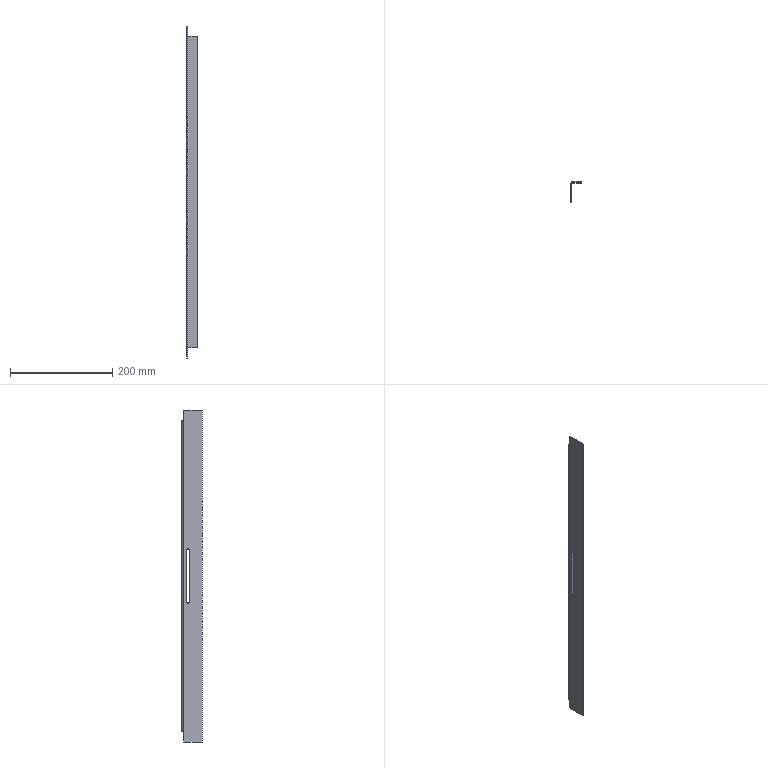Part | SolidWorks | features SMBaseFlange 2, FlatPattern 1, ICE 1, SheetMetal 1 | 1 solid | 21 faces | box 20 x 40 x 649 mm | volume 70699 mm3 | plane 16 | cylinder 5 | commonest cylinder face diameters 6 x3 4 x1 8 x1
STEP:
#1=CARTESIAN_POINT('',(0.,28.,251.5));
#2=VERTEX_POINT('',#1);
#3=CARTESIAN_POINT('',(0.,31.,254.5));
#4=VERTEX_POINT('',#3);
#5=CARTESIAN_POINT('',(0.,28.,254.5));
#6=DIRECTION('',(1.,0.,0.));
#7=DIRECTION('',(0.,0.,-1.));
#8=AXIS2_PLACEMENT_3D('',#5,#6,#7);
#9=CIRCLE('',#8,3.);
#10=EDGE_CURVE('',#2,#4,#9,.T.);
#11=ORIENTED_EDGE('',*,*,#10,.F.);
#12=CARTESIAN_POINT('',(2.,28.,251.5));
#13=VERTEX_POINT('',#12);
#14=CARTESIAN_POINT('',(0.,28.,251.5));
#15=DIRECTION('',(1.,0.,0.));
#16=VECTOR('',#15,1000.);
#17=LINE('',#14,#16);
#18=EDGE_CURVE('',#2,#13,#17,.T.);
#19=ORIENTED_EDGE('',*,*,#18,.T.);
#20=CARTESIAN_POINT('',(2.,31.,254.5));
#21=VERTEX_POINT('',#20);
#22=CARTESIAN_POINT('',(2.,28.,254.5));
#23=DIRECTION('',(1.,0.,0.));
#24=DIRECTION('',(0.,0.,-1.));
#25=AXIS2_PLACEMENT_3D('',#22,#23,#24);
#26=CIRCLE('',#25,3.);
#27=EDGE_CURVE('',#13,#21,#26,.T.);
#28=ORIENTED_EDGE('',*,*,#27,.T.);
#29=CARTESIAN_POINT('',(0.,31.,254.5));
#30=DIRECTION('',(1.,0.,0.));
#31=VECTOR('',#30,1000.);
#32=LINE('',#29,#31);
#33=EDGE_CURVE('',#4,#21,#32,.T.);
#34=ORIENTED_EDGE('',*,*,#33,.F.);
#35=EDGE_LOOP('',(#11,#19,#28,#34));
#36=FACE_OUTER_BOUND('',#35,.T.);
#37=CARTESIAN_POINT('',(0.,28.,254.5));
#38=DIRECTION('',(1.,0.,0.));
#39=DIRECTION('',(0.,0.,-1.));
#40=AXIS2_PLACEMENT_3D('',#37,#38,#39);
#41=CYLINDRICAL_SURFACE('',#40,3.);
#42=ADVANCED_FACE('',(#36),#41,.F.);
#43=CARTESIAN_POINT('',(4.,40.,609.));
#44=VERTEX_POINT('',#43);
#45=CARTESIAN_POINT('',(4.,38.,609.));
#46=VERTEX_POINT('',#45);
#47=CARTESIAN_POINT('',(4.,40.,609.));
#48=DIRECTION('',(0.,-1.,0.));
#49=VECTOR('',#48,1000.);
#50=LINE('',#47,#49);
#51=EDGE_CURVE('',#44,#46,#50,.T.);
#52=ORIENTED_EDGE('',*,*,#51,.F.);
#53=CARTESIAN_POINT('',(0.,36.,609.));
#54=VERTEX_POINT('',#53);
#55=CARTESIAN_POINT('',(4.,36.,609.));
#56=DIRECTION('',(0.,0.,-1.));
#57=DIRECTION('',(1.,0.,0.));
#58=AXIS2_PLACEMENT_3D('',#55,#56,#57);
#59=CIRCLE('',#58,4.);
#60=EDGE_CURVE('',#54,#44,#59,.T.);
#61=ORIENTED_EDGE('',*,*,#60,.F.);
#62=CARTESIAN_POINT('',(2.,36.,609.));
#63=VERTEX_POINT('',#62);
#64=CARTESIAN_POINT('',(2.,36.,609.));
#65=DIRECTION('',(-1.,0.,0.));
#66=VECTOR('',#65,1000.);
#67=LINE('',#64,#66);
#68=EDGE_CURVE('',#63,#54,#67,.T.);
#69=ORIENTED_EDGE('',*,*,#68,.F.);
#70=CARTESIAN_POINT('',(4.,36.,609.));
#71=DIRECTION('',(0.,0.,-1.));
#72=DIRECTION('',(1.,0.,0.));
#73=AXIS2_PLACEMENT_3D('',#70,#71,#72);
#74=CIRCLE('',#73,2.);
#75=EDGE_CURVE('',#63,#46,#74,.T.);
#76=ORIENTED_EDGE('',*,*,#75,.T.);
#77=EDGE_LOOP('',(#52,#61,#69,#76));
#78=FACE_OUTER_BOUND('',#77,.T.);
#79=CARTESIAN_POINT('',(4.,40.,609.));
#80=DIRECTION('',(0.,0.,1.));
#81=DIRECTION('',(1.,0.,0.));
#82=AXIS2_PLACEMENT_3D('',#79,#80,#81);
#83=PLANE('',#82);
#84=ADVANCED_FACE('',(#78),#83,.T.);
#85=CARTESIAN_POINT('',(20.,40.,609.));
#86=VERTEX_POINT('',#85);
#87=CARTESIAN_POINT('',(0.,40.,609.));
#88=DIRECTION('',(1.,0.,0.));
#89=VECTOR('',#88,1000.);
#90=LINE('',#87,#89);
#91=EDGE_CURVE('',#44,#86,#90,.T.);
#92=ORIENTED_EDGE('',*,*,#91,.F.);
#93=ORIENTED_EDGE('',*,*,#51,.T.);
#94=CARTESIAN_POINT('',(20.,38.,609.));
#95=VERTEX_POINT('',#94);
#96=CARTESIAN_POINT('',(0.,38.,609.));
#97=DIRECTION('',(1.,0.,0.));
#98=VECTOR('',#97,1000.);
#99=LINE('',#96,#98);
#100=EDGE_CURVE('',#46,#95,#99,.T.);
#101=ORIENTED_EDGE('',*,*,#100,.T.);
#102=CARTESIAN_POINT('',(20.,40.,609.));
#103=DIRECTION('',(0.,-1.,0.));
#104=VECTOR('',#103,1000.);
#105=LINE('',#102,#104);
#106=EDGE_CURVE('',#86,#95,#105,.T.);
#107=ORIENTED_EDGE('',*,*,#106,.F.);
#108=EDGE_LOOP('',(#92,#93,#101,#107));
#109=FACE_OUTER_BOUND('',#108,.T.);
#110=CARTESIAN_POINT('',(2.,36.,609.));
#111=DIRECTION('',(0.,0.,1.));
#112=DIRECTION('',(1.,0.,0.));
#113=AXIS2_PLACEMENT_3D('',#110,#111,#112);
#114=PLANE('',#113);
#115=ADVANCED_FACE('',(#109),#114,.T.);
#116=CARTESIAN_POINT('',(0.,36.,0.));
#117=VERTEX_POINT('',#116);
#118=CARTESIAN_POINT('',(2.,36.,0.));
#119=VERTEX_POINT('',#118);
#120=CARTESIAN_POINT('',(0.,36.,0.));
#121=DIRECTION('',(1.,0.,0.));
#122=VECTOR('',#121,1000.);
#123=LINE('',#120,#122);
#124=EDGE_CURVE('',#117,#119,#123,.T.);
#125=ORIENTED_EDGE('',*,*,#124,.F.);
#126=CARTESIAN_POINT('',(4.,40.,0.));
#127=VERTEX_POINT('',#126);
#128=CARTESIAN_POINT('',(4.,36.,0.));
#129=DIRECTION('',(0.,0.,-1.));
#130=DIRECTION('',(1.,0.,0.));
#131=AXIS2_PLACEMENT_3D('',#128,#129,#130);
#132=CIRCLE('',#131,4.);
#133=EDGE_CURVE('',#117,#127,#132,.T.);
#134=ORIENTED_EDGE('',*,*,#133,.T.);
#135=CARTESIAN_POINT('',(4.,38.,0.));
#136=VERTEX_POINT('',#135);
#137=CARTESIAN_POINT('',(4.,38.,0.));
#138=DIRECTION('',(0.,1.,0.));
#139=VECTOR('',#138,1000.);
#140=LINE('',#137,#139);
#141=EDGE_CURVE('',#136,#127,#140,.T.);
#142=ORIENTED_EDGE('',*,*,#141,.F.);
#143=CARTESIAN_POINT('',(4.,36.,0.));
#144=DIRECTION('',(0.,0.,-1.));
#145=DIRECTION('',(1.,0.,0.));
#146=AXIS2_PLACEMENT_3D('',#143,#144,#145);
#147=CIRCLE('',#146,2.);
#148=EDGE_CURVE('',#119,#136,#147,.T.);
#149=ORIENTED_EDGE('',*,*,#148,.F.);
#150=EDGE_LOOP('',(#125,#134,#142,#149));
#151=FACE_OUTER_BOUND('',#150,.T.);
#152=CARTESIAN_POINT('',(0.,36.,0.));
#153=DIRECTION('',(0.,0.,-1.));
#154=DIRECTION('',(-1.,0.,0.));
#155=AXIS2_PLACEMENT_3D('',#152,#153,#154);
#156=PLANE('',#155);
#157=ADVANCED_FACE('',(#151),#156,.T.);
#158=CARTESIAN_POINT('',(20.,38.,0.));
#159=VERTEX_POINT('',#158);
#160=CARTESIAN_POINT('',(0.,38.,0.));
#161=DIRECTION('',(1.,0.,0.));
#162=VECTOR('',#161,1000.);
#163=LINE('',#160,#162);
#164=EDGE_CURVE('',#136,#159,#163,.T.);
#165=ORIENTED_EDGE('',*,*,#164,.T.);
#166=CARTESIAN_POINT('',(20.,38.,609.));
#167=DIRECTION('',(0.,0.,-1.));
#168=VECTOR('',#167,1000.);
#169=LINE('',#166,#168);
#170=EDGE_CURVE('',#95,#159,#169,.T.);
#171=ORIENTED_EDGE('',*,*,#170,.F.);
#172=ORIENTED_EDGE('',*,*,#100,.F.);
#173=CARTESIAN_POINT('',(4.,38.,609.));
#174=DIRECTION('',(0.,0.,-1.));
#175=VECTOR('',#174,1000.);
#176=LINE('',#173,#175);
#177=EDGE_CURVE('',#46,#136,#176,.T.);
#178=ORIENTED_EDGE('',*,*,#177,.T.);
#179=EDGE_LOOP('',(#165,#171,#172,#178));
#180=FACE_OUTER_BOUND('',#179,.T.);
#181=CARTESIAN_POINT('',(0.,38.,609.));
#182=DIRECTION('',(0.,1.,0.));
#183=DIRECTION('',(0.,0.,1.));
#184=AXIS2_PLACEMENT_3D('',#181,#182,#183);
#185=PLANE('',#184);
#186=ADVANCED_FACE('',(#180),#185,.F.);
#187=CARTESIAN_POINT('',(20.,40.,0.));
#188=VERTEX_POINT('',#187);
#189=CARTESIAN_POINT('',(20.,40.,0.));
#190=DIRECTION('',(0.,-1.,0.));
#191=VECTOR('',#190,1000.);
#192=LINE('',#189,#191);
#193=EDGE_CURVE('',#188,#159,#192,.T.);
#194=ORIENTED_EDGE('',*,*,#193,.F.);
#195=CARTESIAN_POINT('',(20.,40.,609.));
#196=DIRECTION('',(0.,0.,-1.));
#197=VECTOR('',#196,1000.);
#198=LINE('',#195,#197);
#199=EDGE_CURVE('',#86,#188,#198,.T.);
#200=ORIENTED_EDGE('',*,*,#199,.F.);
#201=ORIENTED_EDGE('',*,*,#106,.T.);
#202=ORIENTED_EDGE('',*,*,#170,.T.);
#203=EDGE_LOOP('',(#194,#200,#201,#202));
#204=FACE_OUTER_BOUND('',#203,.T.);
#205=CARTESIAN_POINT('',(20.,40.,609.));
#206=DIRECTION('',(1.,0.,0.));
#207=DIRECTION('',(0.,0.,-1.));
#208=AXIS2_PLACEMENT_3D('',#205,#206,#207);
#209=PLANE('',#208);
#210=ADVANCED_FACE('',(#204),#209,.T.);
#211=CARTESIAN_POINT('',(0.,40.,0.));
#212=DIRECTION('',(1.,0.,0.));
#213=VECTOR('',#212,1000.);
#214=LINE('',#211,#213);
#215=EDGE_CURVE('',#127,#188,#214,.T.);
#216=ORIENTED_EDGE('',*,*,#215,.F.);
#217=CARTESIAN_POINT('',(4.,40.,609.));
#218=DIRECTION('',(0.,0.,-1.));
#219=VECTOR('',#218,1000.);
#220=LINE('',#217,#219);
#221=EDGE_CURVE('',#44,#127,#220,.T.);
#222=ORIENTED_EDGE('',*,*,#221,.F.);
#223=ORIENTED_EDGE('',*,*,#91,.T.);
#224=ORIENTED_EDGE('',*,*,#199,.T.);
#225=EDGE_LOOP('',(#216,#222,#223,#224));
#226=FACE_OUTER_BOUND('',#225,.T.);
#227=CARTESIAN_POINT('',(0.,40.,609.));
#228=DIRECTION('',(0.,1.,0.));
#229=DIRECTION('',(0.,0.,1.));
#230=AXIS2_PLACEMENT_3D('',#227,#228,#229);
#231=PLANE('',#230);
#232=ADVANCED_FACE('',(#226),#231,.T.);
#233=ORIENTED_EDGE('',*,*,#133,.F.);
#234=CARTESIAN_POINT('',(0.,36.,609.));
#235=DIRECTION('',(0.,0.,-1.));
#236=VECTOR('',#235,1000.);
#237=LINE('',#234,#236);
#238=EDGE_CURVE('',#54,#117,#237,.T.);
#239=ORIENTED_EDGE('',*,*,#238,.F.);
#240=ORIENTED_EDGE('',*,*,#60,.T.);
#241=ORIENTED_EDGE('',*,*,#221,.T.);
#242=EDGE_LOOP('',(#233,#239,#240,#241));
#243=FACE_OUTER_BOUND('',#242,.T.);
#244=CARTESIAN_POINT('',(4.,36.,609.));
#245=DIRECTION('',(0.,0.,-1.));
#246=DIRECTION('',(-1.,0.,0.));
#247=AXIS2_PLACEMENT_3D('',#244,#245,#246);
#248=CYLINDRICAL_SURFACE('',#247,4.);
#249=ADVANCED_FACE('',(#243),#248,.T.);
#250=CARTESIAN_POINT('',(0.,25.,254.5));
#251=VERTEX_POINT('',#250);
#252=CARTESIAN_POINT('',(0.,28.,254.5));
#253=DIRECTION('',(1.,0.,0.));
#254=DIRECTION('',(0.,0.,-1.));
#255=AXIS2_PLACEMENT_3D('',#252,#253,#254);
#256=CIRCLE('',#255,3.);
#257=EDGE_CURVE('',#251,#2,#256,.T.);
#258=ORIENTED_EDGE('',*,*,#257,.T.);
#259=ORIENTED_EDGE('',*,*,#10,.T.);
#260=CARTESIAN_POINT('',(0.,31.,354.5));
#261=VERTEX_POINT('',#260);
#262=CARTESIAN_POINT('',(0.,31.,254.5));
#263=DIRECTION('',(0.,0.,1.));
#264=VECTOR('',#263,1000.);
#265=LINE('',#262,#264);
#266=EDGE_CURVE('',#4,#261,#265,.T.);
#267=ORIENTED_EDGE('',*,*,#266,.T.);
#268=CARTESIAN_POINT('',(0.,25.,354.5));
#269=VERTEX_POINT('',#268);
#270=CARTESIAN_POINT('',(0.,28.,354.5));
#271=DIRECTION('',(1.,0.,0.));
#272=DIRECTION('',(0.,0.,-1.));
#273=AXIS2_PLACEMENT_3D('',#270,#271,#272);
#274=CIRCLE('',#273,3.);
#275=EDGE_CURVE('',#261,#269,#274,.T.);
#276=ORIENTED_EDGE('',*,*,#275,.T.);
#277=CARTESIAN_POINT('',(0.,25.,254.5));
#278=DIRECTION('',(0.,0.,-1.));
#279=VECTOR('',#278,1000.);
#280=LINE('',#277,#279);
#281=EDGE_CURVE('',#269,#251,#280,.T.);
#282=ORIENTED_EDGE('',*,*,#281,.T.);
#283=EDGE_LOOP('',(#258,#259,#267,#276,#282));
#284=FACE_BOUND('',#283,.T.);
#285=ORIENTED_EDGE('',*,*,#238,.T.);
#286=CARTESIAN_POINT('',(0.,36.,-20.));
#287=VERTEX_POINT('',#286);
#288=CARTESIAN_POINT('',(0.,36.,0.));
#289=DIRECTION('',(0.,0.,1.));
#290=VECTOR('',#289,1000.);
#291=LINE('',#288,#290);
#292=EDGE_CURVE('',#287,#117,#291,.T.);
#293=ORIENTED_EDGE('',*,*,#292,.F.);
#294=CARTESIAN_POINT('',(0.,0.,-20.));
#295=VERTEX_POINT('',#294);
#296=CARTESIAN_POINT('',(0.,0.,-20.));
#297=DIRECTION('',(0.,1.,0.));
#298=VECTOR('',#297,1000.);
#299=LINE('',#296,#298);
#300=EDGE_CURVE('',#295,#287,#299,.T.);
#301=ORIENTED_EDGE('',*,*,#300,.F.);
#302=CARTESIAN_POINT('',(0.,0.,629.));
#303=VERTEX_POINT('',#302);
#304=CARTESIAN_POINT('',(0.,0.,609.));
#305=DIRECTION('',(0.,0.,-1.));
#306=VECTOR('',#305,1000.);
#307=LINE('',#304,#306);
#308=EDGE_CURVE('',#303,#295,#307,.T.);
#309=ORIENTED_EDGE('',*,*,#308,.F.);
#310=CARTESIAN_POINT('',(0.,36.,629.));
#311=VERTEX_POINT('',#310);
#312=CARTESIAN_POINT('',(0.,0.,629.));
#313=DIRECTION('',(0.,-1.,0.));
#314=VECTOR('',#313,1000.);
#315=LINE('',#312,#314);
#316=EDGE_CURVE('',#311,#303,#315,.T.);
#317=ORIENTED_EDGE('',*,*,#316,.F.);
#318=CARTESIAN_POINT('',(0.,36.,609.));
#319=DIRECTION('',(0.,0.,1.));
#320=VECTOR('',#319,1000.);
#321=LINE('',#318,#320);
#322=EDGE_CURVE('',#54,#311,#321,.T.);
#323=ORIENTED_EDGE('',*,*,#322,.F.);
#324=EDGE_LOOP('',(#285,#293,#301,#309,#317,#323));
#325=FACE_OUTER_BOUND('',#324,.T.);
#326=CARTESIAN_POINT('',(0.,0.,609.));
#327=DIRECTION('',(-1.,0.,0.));
#328=DIRECTION('',(0.,0.,1.));
#329=AXIS2_PLACEMENT_3D('',#326,#327,#328);
#330=PLANE('',#329);
#331=ADVANCED_FACE('',(#284,#325),#330,.T.);
#332=ORIENTED_EDGE('',*,*,#308,.T.);
#333=CARTESIAN_POINT('',(2.,0.,-20.));
#334=VERTEX_POINT('',#333);
#335=CARTESIAN_POINT('',(0.,0.,-20.));
#336=DIRECTION('',(1.,0.,0.));
#337=VECTOR('',#336,1000.);
#338=LINE('',#335,#337);
#339=EDGE_CURVE('',#295,#334,#338,.T.);
#340=ORIENTED_EDGE('',*,*,#339,.T.);
#341=CARTESIAN_POINT('',(2.,0.,629.));
#342=VERTEX_POINT('',#341);
#343=CARTESIAN_POINT('',(2.,0.,609.));
#344=DIRECTION('',(0.,0.,-1.));
#345=VECTOR('',#344,1000.);
#346=LINE('',#343,#345);
#347=EDGE_CURVE('',#342,#334,#346,.T.);
#348=ORIENTED_EDGE('',*,*,#347,.F.);
#349=CARTESIAN_POINT('',(0.,0.,629.));
#350=DIRECTION('',(1.,0.,0.));
#351=VECTOR('',#350,1000.);
#352=LINE('',#349,#351);
#353=EDGE_CURVE('',#303,#342,#352,.T.);
#354=ORIENTED_EDGE('',*,*,#353,.F.);
#355=EDGE_LOOP('',(#332,#340,#348,#354));
#356=FACE_OUTER_BOUND('',#355,.T.);
#357=CARTESIAN_POINT('',(2.,0.,609.));
#358=DIRECTION('',(0.,-1.,0.));
#359=DIRECTION('',(0.,0.,-1.));
#360=AXIS2_PLACEMENT_3D('',#357,#358,#359);
#361=PLANE('',#360);
#362=ADVANCED_FACE('',(#356),#361,.T.);
#363=CARTESIAN_POINT('',(2.,31.,354.5));
#364=VERTEX_POINT('',#363);
#365=CARTESIAN_POINT('',(2.,31.,254.5));
#366=DIRECTION('',(0.,0.,1.));
#367=VECTOR('',#366,1000.);
#368=LINE('',#365,#367);
#369=EDGE_CURVE('',#21,#364,#368,.T.);
#370=ORIENTED_EDGE('',*,*,#369,.F.);
#371=ORIENTED_EDGE('',*,*,#27,.F.);
#372=CARTESIAN_POINT('',(2.,25.,254.5));
#373=VERTEX_POINT('',#372);
#374=CARTESIAN_POINT('',(2.,28.,254.5));
#375=DIRECTION('',(1.,0.,0.));
#376=DIRECTION('',(0.,0.,-1.));
#377=AXIS2_PLACEMENT_3D('',#374,#375,#376);
#378=CIRCLE('',#377,3.);
#379=EDGE_CURVE('',#373,#13,#378,.T.);
#380=ORIENTED_EDGE('',*,*,#379,.F.);
#381=CARTESIAN_POINT('',(2.,25.,354.5));
#382=VERTEX_POINT('',#381);
#383=CARTESIAN_POINT('',(2.,25.,254.5));
#384=DIRECTION('',(0.,0.,-1.));
#385=VECTOR('',#384,1000.);
#386=LINE('',#383,#385);
#387=EDGE_CURVE('',#382,#373,#386,.T.);
#388=ORIENTED_EDGE('',*,*,#387,.F.);
#389=CARTESIAN_POINT('',(2.,28.,354.5));
#390=DIRECTION('',(1.,0.,0.));
#391=DIRECTION('',(0.,0.,-1.));
#392=AXIS2_PLACEMENT_3D('',#389,#390,#391);
#393=CIRCLE('',#392,3.);
#394=EDGE_CURVE('',#364,#382,#393,.T.);
#395=ORIENTED_EDGE('',*,*,#394,.F.);
#396=EDGE_LOOP('',(#370,#371,#380,#388,#395));
#397=FACE_BOUND('',#396,.T.);
#398=ORIENTED_EDGE('',*,*,#347,.T.);
#399=CARTESIAN_POINT('',(2.,36.,-20.));
#400=VERTEX_POINT('',#399);
#401=CARTESIAN_POINT('',(2.,0.,-20.));
#402=DIRECTION('',(0.,1.,0.));
#403=VECTOR('',#402,1000.);
#404=LINE('',#401,#403);
#405=EDGE_CURVE('',#334,#400,#404,.T.);
#406=ORIENTED_EDGE('',*,*,#405,.T.);
#407=CARTESIAN_POINT('',(2.,36.,0.));
#408=DIRECTION('',(0.,0.,1.));
#409=VECTOR('',#408,1000.);
#410=LINE('',#407,#409);
#411=EDGE_CURVE('',#400,#119,#410,.T.);
#412=ORIENTED_EDGE('',*,*,#411,.T.);
#413=CARTESIAN_POINT('',(2.,36.,609.));
#414=DIRECTION('',(0.,0.,-1.));
#415=VECTOR('',#414,1000.);
#416=LINE('',#413,#415);
#417=EDGE_CURVE('',#63,#119,#416,.T.);
#418=ORIENTED_EDGE('',*,*,#417,.F.);
#419=CARTESIAN_POINT('',(2.,36.,629.));
#420=VERTEX_POINT('',#419);
#421=CARTESIAN_POINT('',(2.,36.,609.));
#422=DIRECTION('',(0.,0.,1.));
#423=VECTOR('',#422,1000.);
#424=LINE('',#421,#423);
#425=EDGE_CURVE('',#63,#420,#424,.T.);
#426=ORIENTED_EDGE('',*,*,#425,.T.);
#427=CARTESIAN_POINT('',(2.,0.,629.));
#428=DIRECTION('',(0.,-1.,0.));
#429=VECTOR('',#428,1000.);
#430=LINE('',#427,#429);
#431=EDGE_CURVE('',#420,#342,#430,.T.);
#432=ORIENTED_EDGE('',*,*,#431,.T.);
#433=EDGE_LOOP('',(#398,#406,#412,#418,#426,#432));
#434=FACE_OUTER_BOUND('',#433,.T.);
#435=CARTESIAN_POINT('',(2.,0.,609.));
#436=DIRECTION('',(-1.,0.,0.));
#437=DIRECTION('',(0.,0.,1.));
#438=AXIS2_PLACEMENT_3D('',#435,#436,#437);
#439=PLANE('',#438);
#440=ADVANCED_FACE('',(#397,#434),#439,.F.);
#441=ORIENTED_EDGE('',*,*,#148,.T.);
#442=ORIENTED_EDGE('',*,*,#177,.F.);
#443=ORIENTED_EDGE('',*,*,#75,.F.);
#444=ORIENTED_EDGE('',*,*,#417,.T.);
#445=EDGE_LOOP('',(#441,#442,#443,#444));
#446=FACE_OUTER_BOUND('',#445,.T.);
#447=CARTESIAN_POINT('',(4.,36.,609.));
#448=DIRECTION('',(0.,0.,-1.));
#449=DIRECTION('',(-1.,0.,0.));
#450=AXIS2_PLACEMENT_3D('',#447,#448,#449);
#451=CYLINDRICAL_SURFACE('',#450,2.);
#452=ADVANCED_FACE('',(#446),#451,.F.);
#453=ORIENTED_EDGE('',*,*,#164,.F.);
#454=ORIENTED_EDGE('',*,*,#141,.T.);
#455=ORIENTED_EDGE('',*,*,#215,.T.);
#456=ORIENTED_EDGE('',*,*,#193,.T.);
#457=EDGE_LOOP('',(#453,#454,#455,#456));
#458=FACE_OUTER_BOUND('',#457,.T.);
#459=CARTESIAN_POINT('',(4.,36.,0.));
#460=DIRECTION('',(0.,0.,1.));
#461=DIRECTION('',(1.,0.,0.));
#462=AXIS2_PLACEMENT_3D('',#459,#460,#461);
#463=PLANE('',#462);
#464=ADVANCED_FACE('',(#458),#463,.F.);
#465=ORIENTED_EDGE('',*,*,#431,.F.);
#466=CARTESIAN_POINT('',(0.,36.,629.));
#467=DIRECTION('',(1.,0.,0.));
#468=VECTOR('',#467,1000.);
#469=LINE('',#466,#468);
#470=EDGE_CURVE('',#311,#420,#469,.T.);
#471=ORIENTED_EDGE('',*,*,#470,.F.);
#472=ORIENTED_EDGE('',*,*,#316,.T.);
#473=ORIENTED_EDGE('',*,*,#353,.T.);
#474=EDGE_LOOP('',(#465,#471,#472,#473));
#475=FACE_OUTER_BOUND('',#474,.T.);
#476=CARTESIAN_POINT('',(0.,0.,629.));
#477=DIRECTION('',(0.,0.,1.));
#478=DIRECTION('',(1.,0.,0.));
#479=AXIS2_PLACEMENT_3D('',#476,#477,#478);
#480=PLANE('',#479);
#481=ADVANCED_FACE('',(#475),#480,.T.);
#482=ORIENTED_EDGE('',*,*,#425,.F.);
#483=ORIENTED_EDGE('',*,*,#68,.T.);
#484=ORIENTED_EDGE('',*,*,#322,.T.);
#485=ORIENTED_EDGE('',*,*,#470,.T.);
#486=EDGE_LOOP('',(#482,#483,#484,#485));
#487=FACE_OUTER_BOUND('',#486,.T.);
#488=CARTESIAN_POINT('',(0.,36.,609.));
#489=DIRECTION('',(0.,1.,0.));
#490=DIRECTION('',(0.,0.,1.));
#491=AXIS2_PLACEMENT_3D('',#488,#489,#490);
#492=PLANE('',#491);
#493=ADVANCED_FACE('',(#487),#492,.T.);
#494=ORIENTED_EDGE('',*,*,#411,.F.);
#495=CARTESIAN_POINT('',(0.,36.,-20.));
#496=DIRECTION('',(1.,0.,0.));
#497=VECTOR('',#496,1000.);
#498=LINE('',#495,#497);
#499=EDGE_CURVE('',#287,#400,#498,.T.);
#500=ORIENTED_EDGE('',*,*,#499,.F.);
#501=ORIENTED_EDGE('',*,*,#292,.T.);
#502=ORIENTED_EDGE('',*,*,#124,.T.);
#503=EDGE_LOOP('',(#494,#500,#501,#502));
#504=FACE_OUTER_BOUND('',#503,.T.);
#505=CARTESIAN_POINT('',(0.,36.,0.));
#506=DIRECTION('',(0.,1.,0.));
#507=DIRECTION('',(0.,0.,1.));
#508=AXIS2_PLACEMENT_3D('',#505,#506,#507);
#509=PLANE('',#508);
#510=ADVANCED_FACE('',(#504),#509,.T.);
#511=ORIENTED_EDGE('',*,*,#405,.F.);
#512=ORIENTED_EDGE('',*,*,#339,.F.);
#513=ORIENTED_EDGE('',*,*,#300,.T.);
#514=ORIENTED_EDGE('',*,*,#499,.T.);
#515=EDGE_LOOP('',(#511,#512,#513,#514));
#516=FACE_OUTER_BOUND('',#515,.T.);
#517=CARTESIAN_POINT('',(0.,0.,-20.));
#518=DIRECTION('',(0.,0.,-1.));
#519=DIRECTION('',(-1.,0.,0.));
#520=AXIS2_PLACEMENT_3D('',#517,#518,#519);
#521=PLANE('',#520);
#522=ADVANCED_FACE('',(#516),#521,.T.);
#523=ORIENTED_EDGE('',*,*,#18,.F.);
#524=ORIENTED_EDGE('',*,*,#257,.F.);
#525=CARTESIAN_POINT('',(0.,25.,254.5));
#526=DIRECTION('',(1.,0.,0.));
#527=VECTOR('',#526,1000.);
#528=LINE('',#525,#527);
#529=EDGE_CURVE('',#251,#373,#528,.T.);
#530=ORIENTED_EDGE('',*,*,#529,.T.);
#531=ORIENTED_EDGE('',*,*,#379,.T.);
#532=EDGE_LOOP('',(#523,#524,#530,#531));
#533=FACE_OUTER_BOUND('',#532,.T.);
#534=CARTESIAN_POINT('',(0.,28.,254.5));
#535=DIRECTION('',(1.,0.,0.));
#536=DIRECTION('',(0.,0.,-1.));
#537=AXIS2_PLACEMENT_3D('',#534,#535,#536);
#538=CYLINDRICAL_SURFACE('',#537,3.);
#539=ADVANCED_FACE('',(#533),#538,.F.);
#540=ORIENTED_EDGE('',*,*,#387,.T.);
#541=ORIENTED_EDGE('',*,*,#529,.F.);
#542=ORIENTED_EDGE('',*,*,#281,.F.);
#543=CARTESIAN_POINT('',(0.,25.,354.5));
#544=DIRECTION('',(1.,0.,0.));
#545=VECTOR('',#544,1000.);
#546=LINE('',#543,#545);
#547=EDGE_CURVE('',#269,#382,#546,.T.);
#548=ORIENTED_EDGE('',*,*,#547,.T.);
#549=EDGE_LOOP('',(#540,#541,#542,#548));
#550=FACE_OUTER_BOUND('',#549,.T.);
#551=CARTESIAN_POINT('',(0.,25.,254.5));
#552=DIRECTION('',(0.,-1.,0.));
#553=DIRECTION('',(0.,0.,-1.));
#554=AXIS2_PLACEMENT_3D('',#551,#552,#553);
#555=PLANE('',#554);
#556=ADVANCED_FACE('',(#550),#555,.F.);
#557=ORIENTED_EDGE('',*,*,#394,.T.);
#558=ORIENTED_EDGE('',*,*,#547,.F.);
#559=ORIENTED_EDGE('',*,*,#275,.F.);
#560=CARTESIAN_POINT('',(0.,31.,354.5));
#561=DIRECTION('',(1.,0.,0.));
#562=VECTOR('',#561,1000.);
#563=LINE('',#560,#562);
#564=EDGE_CURVE('',#261,#364,#563,.T.);
#565=ORIENTED_EDGE('',*,*,#564,.T.);
#566=EDGE_LOOP('',(#557,#558,#559,#565));
#567=FACE_OUTER_BOUND('',#566,.T.);
#568=CARTESIAN_POINT('',(0.,28.,354.5));
#569=DIRECTION('',(1.,0.,0.));
#570=DIRECTION('',(0.,0.,-1.));
#571=AXIS2_PLACEMENT_3D('',#568,#569,#570);
#572=CYLINDRICAL_SURFACE('',#571,3.);
#573=ADVANCED_FACE('',(#567),#572,.F.);
#574=ORIENTED_EDGE('',*,*,#369,.T.);
#575=ORIENTED_EDGE('',*,*,#564,.F.);
#576=ORIENTED_EDGE('',*,*,#266,.F.);
#577=ORIENTED_EDGE('',*,*,#33,.T.);
#578=EDGE_LOOP('',(#574,#575,#576,#577));
#579=FACE_OUTER_BOUND('',#578,.T.);
#580=CARTESIAN_POINT('',(0.,31.,254.5));
#581=DIRECTION('',(0.,1.,0.));
#582=DIRECTION('',(0.,0.,1.));
#583=AXIS2_PLACEMENT_3D('',#580,#581,#582);
#584=PLANE('',#583);
#585=ADVANCED_FACE('',(#579),#584,.F.);
#586=CLOSED_SHELL('',(#42,#84,#115,#157,#186,#210,#232,#249,#331,#362,#440,#452,#464,#481,#493,#510,#522,#539,#556,#573,#585));
#587=MANIFOLD_SOLID_BREP('',#586);
#588=CARTESIAN_POINT('',(0.,0.,0.));
#589=DIRECTION('',(0.,0.,1.));
#590=DIRECTION('',(1.,0.,0.));
#591=AXIS2_PLACEMENT_3D('',#588,#589,#590);
#592=(LENGTH_UNIT()NAMED_UNIT(*)SI_UNIT(.MILLI.,.METRE.));
#593=UNCERTAINTY_MEASURE_WITH_UNIT(LENGTH_MEASURE(0.00001),#592,'','');
#594=(NAMED_UNIT(*)PLANE_ANGLE_UNIT()SI_UNIT($,.RADIAN.));
#595=(NAMED_UNIT(*)SI_UNIT($,.STERADIAN.)SOLID_ANGLE_UNIT());
#596=(GEOMETRIC_REPRESENTATION_CONTEXT(3)GLOBAL_UNCERTAINTY_ASSIGNED_CONTEXT((#593))GLOBAL_UNIT_ASSIGNED_CONTEXT((#592,#594,#595))REPRESENTATION_CONTEXT('',''));
#597=ADVANCED_BREP_SHAPE_REPRESENTATION('',(#587,#591),#596);